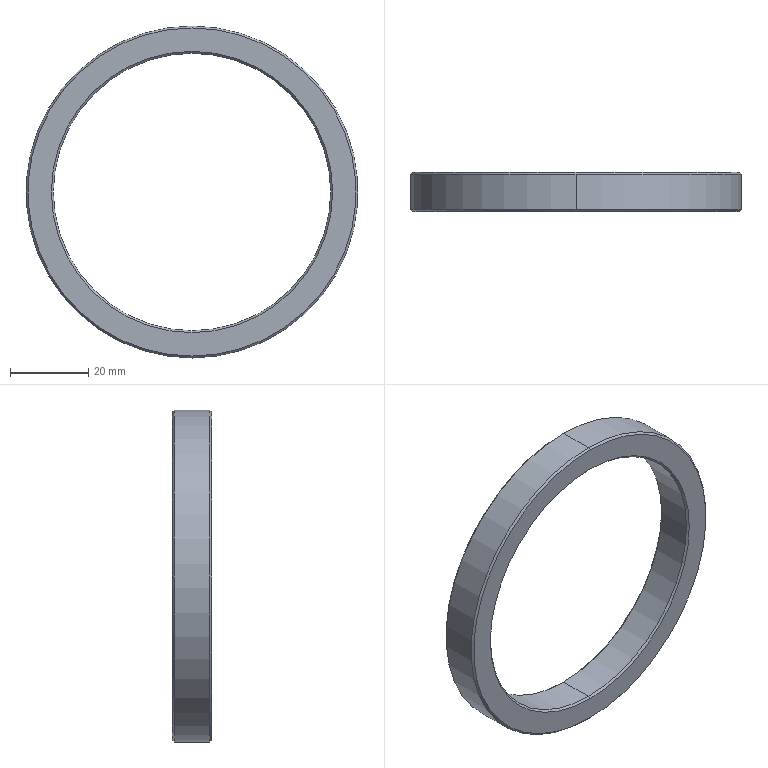Part | SolidWorks | features Chamfer 1, Extrusion 1 | 1 solid | 14 faces | box 85 x 10 x 85 mm | volume 17031 mm3 | cone 8 | cylinder 4 | plane 2 | commonest cylinder face diameters 71 x2 85 x2
STEP:
#1=CARTESIAN_POINT('',(0.,0.5,35.5));
#2=VERTEX_POINT('',#1);
#3=CARTESIAN_POINT('',(0.,0.5,-35.5));
#4=VERTEX_POINT('',#3);
#5=CARTESIAN_POINT('',(0.,0.5,0.));
#6=DIRECTION('',(0.,-1.,0.));
#7=DIRECTION('',(0.,0.,1.));
#8=AXIS2_PLACEMENT_3D('',#5,#6,#7);
#9=CIRCLE('',#8,35.5);
#10=EDGE_CURVE('',#2,#4,#9,.T.);
#11=ORIENTED_EDGE('',*,*,#10,.F.);
#12=CARTESIAN_POINT('',(0.,0.,36.));
#13=VERTEX_POINT('',#12);
#14=CARTESIAN_POINT('',(0.,0.,36.));
#15=DIRECTION('',(0.,-0.7071,0.7071));
#16=VECTOR('',#15,1000.);
#17=LINE('',#14,#16);
#18=EDGE_CURVE('',#2,#13,#17,.T.);
#19=ORIENTED_EDGE('',*,*,#18,.T.);
#20=CARTESIAN_POINT('',(0.,0.,-36.));
#21=VERTEX_POINT('',#20);
#22=CARTESIAN_POINT('',(0.,0.,0.));
#23=DIRECTION('',(0.,1.,0.));
#24=DIRECTION('',(0.,0.,1.));
#25=AXIS2_PLACEMENT_3D('',#22,#23,#24);
#26=CIRCLE('',#25,36.);
#27=EDGE_CURVE('',#21,#13,#26,.T.);
#28=ORIENTED_EDGE('',*,*,#27,.F.);
#29=CARTESIAN_POINT('',(0.,0.,-36.));
#30=DIRECTION('',(0.,-0.7071,-0.7071));
#31=VECTOR('',#30,1000.);
#32=LINE('',#29,#31);
#33=EDGE_CURVE('',#4,#21,#32,.T.);
#34=ORIENTED_EDGE('',*,*,#33,.F.);
#35=EDGE_LOOP('',(#11,#19,#28,#34));
#36=FACE_OUTER_BOUND('',#35,.T.);
#37=CARTESIAN_POINT('',(0.,0.,0.));
#38=DIRECTION('',(0.,-1.,0.));
#39=DIRECTION('',(0.,0.,-1.));
#40=AXIS2_PLACEMENT_3D('',#37,#38,#39);
#41=CONICAL_SURFACE('',#40,36.,0.7854);
#42=ADVANCED_FACE('',(#36),#41,.F.);
#43=CARTESIAN_POINT('',(0.,9.5,-35.5));
#44=VERTEX_POINT('',#43);
#45=CARTESIAN_POINT('',(0.,9.5,35.5));
#46=VERTEX_POINT('',#45);
#47=CARTESIAN_POINT('',(0.,9.5,0.));
#48=DIRECTION('',(0.,1.,0.));
#49=DIRECTION('',(0.,0.,1.));
#50=AXIS2_PLACEMENT_3D('',#47,#48,#49);
#51=CIRCLE('',#50,35.5);
#52=EDGE_CURVE('',#44,#46,#51,.T.);
#53=ORIENTED_EDGE('',*,*,#52,.F.);
#54=CARTESIAN_POINT('',(0.,10.,-36.));
#55=VERTEX_POINT('',#54);
#56=CARTESIAN_POINT('',(0.,9.5,-35.5));
#57=DIRECTION('',(0.,0.7071,-0.7071));
#58=VECTOR('',#57,1000.);
#59=LINE('',#56,#58);
#60=EDGE_CURVE('',#44,#55,#59,.T.);
#61=ORIENTED_EDGE('',*,*,#60,.T.);
#62=CARTESIAN_POINT('',(0.,10.,36.));
#63=VERTEX_POINT('',#62);
#64=CARTESIAN_POINT('',(0.,10.,0.));
#65=DIRECTION('',(0.,-1.,0.));
#66=DIRECTION('',(0.,0.,1.));
#67=AXIS2_PLACEMENT_3D('',#64,#65,#66);
#68=CIRCLE('',#67,36.);
#69=EDGE_CURVE('',#63,#55,#68,.T.);
#70=ORIENTED_EDGE('',*,*,#69,.F.);
#71=CARTESIAN_POINT('',(0.,9.5,35.5));
#72=DIRECTION('',(0.,0.7071,0.7071));
#73=VECTOR('',#72,1000.);
#74=LINE('',#71,#73);
#75=EDGE_CURVE('',#46,#63,#74,.T.);
#76=ORIENTED_EDGE('',*,*,#75,.F.);
#77=EDGE_LOOP('',(#53,#61,#70,#76));
#78=FACE_OUTER_BOUND('',#77,.T.);
#79=CARTESIAN_POINT('',(0.,9.5,0.));
#80=DIRECTION('',(0.,1.,0.));
#81=DIRECTION('',(0.,0.,1.));
#82=AXIS2_PLACEMENT_3D('',#79,#80,#81);
#83=CONICAL_SURFACE('',#82,35.5,0.7854);
#84=ADVANCED_FACE('',(#78),#83,.F.);
#85=CARTESIAN_POINT('',(0.,0.,-42.));
#86=VERTEX_POINT('',#85);
#87=CARTESIAN_POINT('',(0.,0.,42.));
#88=VERTEX_POINT('',#87);
#89=CARTESIAN_POINT('',(0.,0.,0.));
#90=DIRECTION('',(0.,-1.,0.));
#91=DIRECTION('',(0.,0.,1.));
#92=AXIS2_PLACEMENT_3D('',#89,#90,#91);
#93=CIRCLE('',#92,42.);
#94=EDGE_CURVE('',#86,#88,#93,.T.);
#95=ORIENTED_EDGE('',*,*,#94,.F.);
#96=CARTESIAN_POINT('',(0.,0.5,-42.5));
#97=VERTEX_POINT('',#96);
#98=CARTESIAN_POINT('',(0.,0.5,-42.5));
#99=DIRECTION('',(0.,0.7071,-0.7071));
#100=VECTOR('',#99,1000.);
#101=LINE('',#98,#100);
#102=EDGE_CURVE('',#86,#97,#101,.T.);
#103=ORIENTED_EDGE('',*,*,#102,.T.);
#104=CARTESIAN_POINT('',(0.,0.5,42.5));
#105=VERTEX_POINT('',#104);
#106=CARTESIAN_POINT('',(0.,0.5,0.));
#107=DIRECTION('',(0.,1.,0.));
#108=DIRECTION('',(0.,0.,1.));
#109=AXIS2_PLACEMENT_3D('',#106,#107,#108);
#110=CIRCLE('',#109,42.5);
#111=EDGE_CURVE('',#105,#97,#110,.T.);
#112=ORIENTED_EDGE('',*,*,#111,.F.);
#113=CARTESIAN_POINT('',(0.,0.5,42.5));
#114=DIRECTION('',(0.,0.7071,0.7071));
#115=VECTOR('',#114,1000.);
#116=LINE('',#113,#115);
#117=EDGE_CURVE('',#88,#105,#116,.T.);
#118=ORIENTED_EDGE('',*,*,#117,.F.);
#119=EDGE_LOOP('',(#95,#103,#112,#118));
#120=FACE_OUTER_BOUND('',#119,.T.);
#121=CARTESIAN_POINT('',(0.,0.5,0.));
#122=DIRECTION('',(0.,1.,0.));
#123=DIRECTION('',(0.,0.,1.));
#124=AXIS2_PLACEMENT_3D('',#121,#122,#123);
#125=CONICAL_SURFACE('',#124,42.5,0.7854);
#126=ADVANCED_FACE('',(#120),#125,.T.);
#127=CARTESIAN_POINT('',(0.,10.,42.));
#128=VERTEX_POINT('',#127);
#129=CARTESIAN_POINT('',(0.,10.,-42.));
#130=VERTEX_POINT('',#129);
#131=CARTESIAN_POINT('',(0.,10.,0.));
#132=DIRECTION('',(0.,1.,0.));
#133=DIRECTION('',(0.,0.,1.));
#134=AXIS2_PLACEMENT_3D('',#131,#132,#133);
#135=CIRCLE('',#134,42.);
#136=EDGE_CURVE('',#128,#130,#135,.T.);
#137=ORIENTED_EDGE('',*,*,#136,.F.);
#138=CARTESIAN_POINT('',(0.,9.5,42.5));
#139=VERTEX_POINT('',#138);
#140=CARTESIAN_POINT('',(0.,10.,42.));
#141=DIRECTION('',(0.,-0.7071,0.7071));
#142=VECTOR('',#141,1000.);
#143=LINE('',#140,#142);
#144=EDGE_CURVE('',#128,#139,#143,.T.);
#145=ORIENTED_EDGE('',*,*,#144,.T.);
#146=CARTESIAN_POINT('',(0.,9.5,-42.5));
#147=VERTEX_POINT('',#146);
#148=CARTESIAN_POINT('',(0.,9.5,0.));
#149=DIRECTION('',(0.,-1.,0.));
#150=DIRECTION('',(0.,0.,1.));
#151=AXIS2_PLACEMENT_3D('',#148,#149,#150);
#152=CIRCLE('',#151,42.5);
#153=EDGE_CURVE('',#147,#139,#152,.T.);
#154=ORIENTED_EDGE('',*,*,#153,.F.);
#155=CARTESIAN_POINT('',(0.,10.,-42.));
#156=DIRECTION('',(0.,-0.7071,-0.7071));
#157=VECTOR('',#156,1000.);
#158=LINE('',#155,#157);
#159=EDGE_CURVE('',#130,#147,#158,.T.);
#160=ORIENTED_EDGE('',*,*,#159,.F.);
#161=EDGE_LOOP('',(#137,#145,#154,#160));
#162=FACE_OUTER_BOUND('',#161,.T.);
#163=CARTESIAN_POINT('',(0.,10.,0.));
#164=DIRECTION('',(0.,-1.,0.));
#165=DIRECTION('',(0.,0.,-1.));
#166=AXIS2_PLACEMENT_3D('',#163,#164,#165);
#167=CONICAL_SURFACE('',#166,42.,0.7854);
#168=ADVANCED_FACE('',(#162),#167,.T.);
#169=ORIENTED_EDGE('',*,*,#52,.T.);
#170=CARTESIAN_POINT('',(0.,10.,35.5));
#171=DIRECTION('',(0.,-1.,0.));
#172=VECTOR('',#171,1000.);
#173=LINE('',#170,#172);
#174=EDGE_CURVE('',#46,#2,#173,.T.);
#175=ORIENTED_EDGE('',*,*,#174,.T.);
#176=ORIENTED_EDGE('',*,*,#10,.T.);
#177=CARTESIAN_POINT('',(0.,10.,-35.5));
#178=DIRECTION('',(0.,-1.,0.));
#179=VECTOR('',#178,1000.);
#180=LINE('',#177,#179);
#181=EDGE_CURVE('',#44,#4,#180,.T.);
#182=ORIENTED_EDGE('',*,*,#181,.F.);
#183=EDGE_LOOP('',(#169,#175,#176,#182));
#184=FACE_OUTER_BOUND('',#183,.T.);
#185=CARTESIAN_POINT('',(0.,10.,0.));
#186=DIRECTION('',(0.,-1.,0.));
#187=DIRECTION('',(0.,0.,-1.));
#188=AXIS2_PLACEMENT_3D('',#185,#186,#187);
#189=CYLINDRICAL_SURFACE('',#188,35.5);
#190=ADVANCED_FACE('',(#184),#189,.F.);
#191=ORIENTED_EDGE('',*,*,#153,.T.);
#192=CARTESIAN_POINT('',(0.,10.,42.5));
#193=DIRECTION('',(0.,-1.,0.));
#194=VECTOR('',#193,1000.);
#195=LINE('',#192,#194);
#196=EDGE_CURVE('',#139,#105,#195,.T.);
#197=ORIENTED_EDGE('',*,*,#196,.T.);
#198=ORIENTED_EDGE('',*,*,#111,.T.);
#199=CARTESIAN_POINT('',(0.,10.,-42.5));
#200=DIRECTION('',(0.,-1.,0.));
#201=VECTOR('',#200,1000.);
#202=LINE('',#199,#201);
#203=EDGE_CURVE('',#147,#97,#202,.T.);
#204=ORIENTED_EDGE('',*,*,#203,.F.);
#205=EDGE_LOOP('',(#191,#197,#198,#204));
#206=FACE_OUTER_BOUND('',#205,.T.);
#207=CARTESIAN_POINT('',(0.,10.,0.));
#208=DIRECTION('',(0.,-1.,0.));
#209=DIRECTION('',(0.,0.,-1.));
#210=AXIS2_PLACEMENT_3D('',#207,#208,#209);
#211=CYLINDRICAL_SURFACE('',#210,42.5);
#212=ADVANCED_FACE('',(#206),#211,.T.);
#213=CARTESIAN_POINT('',(0.,10.,0.));
#214=DIRECTION('',(0.,1.,0.));
#215=DIRECTION('',(0.,0.,1.));
#216=AXIS2_PLACEMENT_3D('',#213,#214,#215);
#217=CIRCLE('',#216,42.);
#218=EDGE_CURVE('',#130,#128,#217,.T.);
#219=ORIENTED_EDGE('',*,*,#218,.T.);
#220=ORIENTED_EDGE('',*,*,#136,.T.);
#221=EDGE_LOOP('',(#219,#220));
#222=FACE_OUTER_BOUND('',#221,.T.);
#223=ORIENTED_EDGE('',*,*,#69,.T.);
#224=CARTESIAN_POINT('',(0.,10.,0.));
#225=DIRECTION('',(0.,-1.,0.));
#226=DIRECTION('',(0.,0.,1.));
#227=AXIS2_PLACEMENT_3D('',#224,#225,#226);
#228=CIRCLE('',#227,36.);
#229=EDGE_CURVE('',#55,#63,#228,.T.);
#230=ORIENTED_EDGE('',*,*,#229,.T.);
#231=EDGE_LOOP('',(#223,#230));
#232=FACE_BOUND('',#231,.T.);
#233=CARTESIAN_POINT('',(0.,10.,0.));
#234=DIRECTION('',(0.,1.,0.));
#235=DIRECTION('',(0.,0.,1.));
#236=AXIS2_PLACEMENT_3D('',#233,#234,#235);
#237=PLANE('',#236);
#238=ADVANCED_FACE('',(#222,#232),#237,.T.);
#239=CARTESIAN_POINT('',(0.,0.,0.));
#240=DIRECTION('',(0.,-1.,0.));
#241=DIRECTION('',(0.,0.,1.));
#242=AXIS2_PLACEMENT_3D('',#239,#240,#241);
#243=CIRCLE('',#242,42.);
#244=EDGE_CURVE('',#88,#86,#243,.T.);
#245=ORIENTED_EDGE('',*,*,#244,.T.);
#246=ORIENTED_EDGE('',*,*,#94,.T.);
#247=EDGE_LOOP('',(#245,#246));
#248=FACE_OUTER_BOUND('',#247,.T.);
#249=ORIENTED_EDGE('',*,*,#27,.T.);
#250=CARTESIAN_POINT('',(0.,0.,0.));
#251=DIRECTION('',(0.,1.,0.));
#252=DIRECTION('',(0.,0.,1.));
#253=AXIS2_PLACEMENT_3D('',#250,#251,#252);
#254=CIRCLE('',#253,36.);
#255=EDGE_CURVE('',#13,#21,#254,.T.);
#256=ORIENTED_EDGE('',*,*,#255,.T.);
#257=EDGE_LOOP('',(#249,#256));
#258=FACE_BOUND('',#257,.T.);
#259=CARTESIAN_POINT('',(0.,0.,0.));
#260=DIRECTION('',(0.,1.,0.));
#261=DIRECTION('',(0.,0.,1.));
#262=AXIS2_PLACEMENT_3D('',#259,#260,#261);
#263=PLANE('',#262);
#264=ADVANCED_FACE('',(#248,#258),#263,.F.);
#265=ORIENTED_EDGE('',*,*,#196,.F.);
#266=CARTESIAN_POINT('',(0.,9.5,0.));
#267=DIRECTION('',(0.,-1.,0.));
#268=DIRECTION('',(0.,0.,1.));
#269=AXIS2_PLACEMENT_3D('',#266,#267,#268);
#270=CIRCLE('',#269,42.5);
#271=EDGE_CURVE('',#139,#147,#270,.T.);
#272=ORIENTED_EDGE('',*,*,#271,.T.);
#273=ORIENTED_EDGE('',*,*,#203,.T.);
#274=CARTESIAN_POINT('',(0.,0.5,0.));
#275=DIRECTION('',(0.,1.,0.));
#276=DIRECTION('',(0.,0.,1.));
#277=AXIS2_PLACEMENT_3D('',#274,#275,#276);
#278=CIRCLE('',#277,42.5);
#279=EDGE_CURVE('',#97,#105,#278,.T.);
#280=ORIENTED_EDGE('',*,*,#279,.T.);
#281=EDGE_LOOP('',(#265,#272,#273,#280));
#282=FACE_OUTER_BOUND('',#281,.T.);
#283=CARTESIAN_POINT('',(0.,10.,0.));
#284=DIRECTION('',(0.,-1.,0.));
#285=DIRECTION('',(0.,0.,-1.));
#286=AXIS2_PLACEMENT_3D('',#283,#284,#285);
#287=CYLINDRICAL_SURFACE('',#286,42.5);
#288=ADVANCED_FACE('',(#282),#287,.T.);
#289=ORIENTED_EDGE('',*,*,#174,.F.);
#290=CARTESIAN_POINT('',(0.,9.5,0.));
#291=DIRECTION('',(0.,1.,0.));
#292=DIRECTION('',(0.,0.,1.));
#293=AXIS2_PLACEMENT_3D('',#290,#291,#292);
#294=CIRCLE('',#293,35.5);
#295=EDGE_CURVE('',#46,#44,#294,.T.);
#296=ORIENTED_EDGE('',*,*,#295,.T.);
#297=ORIENTED_EDGE('',*,*,#181,.T.);
#298=CARTESIAN_POINT('',(0.,0.5,0.));
#299=DIRECTION('',(0.,-1.,0.));
#300=DIRECTION('',(0.,0.,1.));
#301=AXIS2_PLACEMENT_3D('',#298,#299,#300);
#302=CIRCLE('',#301,35.5);
#303=EDGE_CURVE('',#4,#2,#302,.T.);
#304=ORIENTED_EDGE('',*,*,#303,.T.);
#305=EDGE_LOOP('',(#289,#296,#297,#304));
#306=FACE_OUTER_BOUND('',#305,.T.);
#307=CARTESIAN_POINT('',(0.,10.,0.));
#308=DIRECTION('',(0.,-1.,0.));
#309=DIRECTION('',(0.,0.,-1.));
#310=AXIS2_PLACEMENT_3D('',#307,#308,#309);
#311=CYLINDRICAL_SURFACE('',#310,35.5);
#312=ADVANCED_FACE('',(#306),#311,.F.);
#313=ORIENTED_EDGE('',*,*,#144,.F.);
#314=ORIENTED_EDGE('',*,*,#218,.F.);
#315=ORIENTED_EDGE('',*,*,#159,.T.);
#316=ORIENTED_EDGE('',*,*,#271,.F.);
#317=EDGE_LOOP('',(#313,#314,#315,#316));
#318=FACE_OUTER_BOUND('',#317,.T.);
#319=CARTESIAN_POINT('',(0.,10.,0.));
#320=DIRECTION('',(0.,-1.,0.));
#321=DIRECTION('',(0.,0.,-1.));
#322=AXIS2_PLACEMENT_3D('',#319,#320,#321);
#323=CONICAL_SURFACE('',#322,42.,0.7854);
#324=ADVANCED_FACE('',(#318),#323,.T.);
#325=ORIENTED_EDGE('',*,*,#102,.F.);
#326=ORIENTED_EDGE('',*,*,#244,.F.);
#327=ORIENTED_EDGE('',*,*,#117,.T.);
#328=ORIENTED_EDGE('',*,*,#279,.F.);
#329=EDGE_LOOP('',(#325,#326,#327,#328));
#330=FACE_OUTER_BOUND('',#329,.T.);
#331=CARTESIAN_POINT('',(0.,0.5,0.));
#332=DIRECTION('',(0.,1.,0.));
#333=DIRECTION('',(0.,0.,1.));
#334=AXIS2_PLACEMENT_3D('',#331,#332,#333);
#335=CONICAL_SURFACE('',#334,42.5,0.7854);
#336=ADVANCED_FACE('',(#330),#335,.T.);
#337=ORIENTED_EDGE('',*,*,#60,.F.);
#338=ORIENTED_EDGE('',*,*,#295,.F.);
#339=ORIENTED_EDGE('',*,*,#75,.T.);
#340=ORIENTED_EDGE('',*,*,#229,.F.);
#341=EDGE_LOOP('',(#337,#338,#339,#340));
#342=FACE_OUTER_BOUND('',#341,.T.);
#343=CARTESIAN_POINT('',(0.,9.5,0.));
#344=DIRECTION('',(0.,1.,0.));
#345=DIRECTION('',(0.,0.,1.));
#346=AXIS2_PLACEMENT_3D('',#343,#344,#345);
#347=CONICAL_SURFACE('',#346,35.5,0.7854);
#348=ADVANCED_FACE('',(#342),#347,.F.);
#349=ORIENTED_EDGE('',*,*,#18,.F.);
#350=ORIENTED_EDGE('',*,*,#303,.F.);
#351=ORIENTED_EDGE('',*,*,#33,.T.);
#352=ORIENTED_EDGE('',*,*,#255,.F.);
#353=EDGE_LOOP('',(#349,#350,#351,#352));
#354=FACE_OUTER_BOUND('',#353,.T.);
#355=CARTESIAN_POINT('',(0.,0.,0.));
#356=DIRECTION('',(0.,-1.,0.));
#357=DIRECTION('',(0.,0.,-1.));
#358=AXIS2_PLACEMENT_3D('',#355,#356,#357);
#359=CONICAL_SURFACE('',#358,36.,0.7854);
#360=ADVANCED_FACE('',(#354),#359,.F.);
#361=CLOSED_SHELL('',(#42,#84,#126,#168,#190,#212,#238,#264,#288,#312,#324,#336,#348,#360));
#362=MANIFOLD_SOLID_BREP('',#361);
#363=CARTESIAN_POINT('',(0.,0.,0.));
#364=DIRECTION('',(0.,0.,1.));
#365=DIRECTION('',(1.,0.,0.));
#366=AXIS2_PLACEMENT_3D('',#363,#364,#365);
#367=(LENGTH_UNIT()NAMED_UNIT(*)SI_UNIT(.MILLI.,.METRE.));
#368=UNCERTAINTY_MEASURE_WITH_UNIT(LENGTH_MEASURE(0.00001),#367,'','');
#369=(NAMED_UNIT(*)PLANE_ANGLE_UNIT()SI_UNIT($,.RADIAN.));
#370=(NAMED_UNIT(*)SI_UNIT($,.STERADIAN.)SOLID_ANGLE_UNIT());
#371=(GEOMETRIC_REPRESENTATION_CONTEXT(3)GLOBAL_UNCERTAINTY_ASSIGNED_CONTEXT((#368))GLOBAL_UNIT_ASSIGNED_CONTEXT((#367,#369,#370))REPRESENTATION_CONTEXT('',''));
#372=ADVANCED_BREP_SHAPE_REPRESENTATION('',(#362,#366),#371);